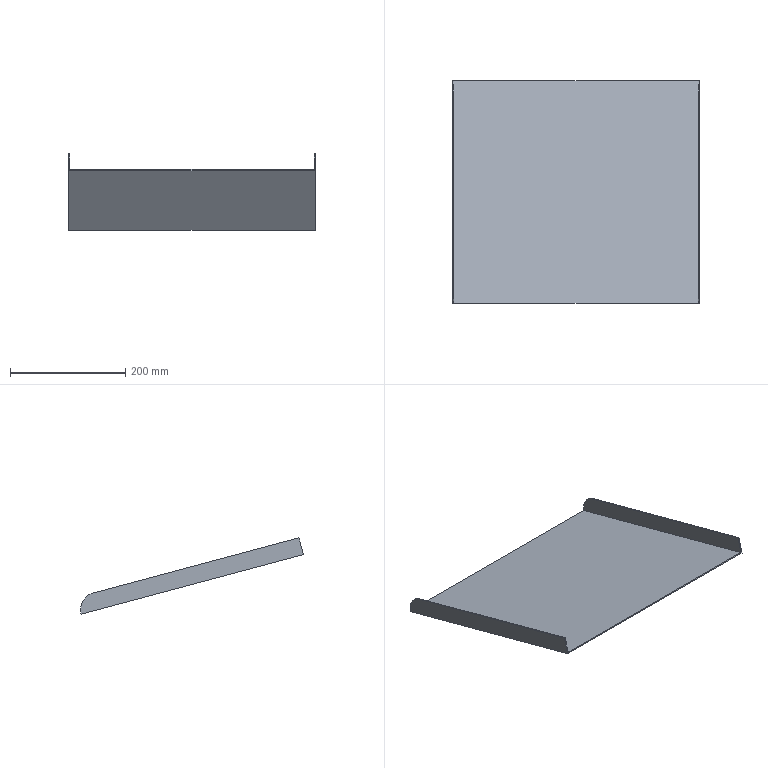Part | NX | features solid 2 | 1 solid | 12 faces | box 428.583 x 387.393 x 132.505 mm | volume 386894 mm3 | plane 10 | cylinder 2 | commonest cylinder face diameters 60 x2
STEP:
#1=CARTESIAN_POINT('',(-915.1,751.036,-491.717));
#2=VERTEX_POINT('',#1);
#3=CARTESIAN_POINT('',(-915.1,1137.342,-595.228));
#4=VERTEX_POINT('',#3);
#5=CARTESIAN_POINT('',(-915.1,973.199,-551.246));
#6=DIRECTION('',(0.,0.9659,-0.2588));
#7=VECTOR('',#6,1000.);
#8=LINE('',#5,#7);
#9=EDGE_CURVE('',#2,#4,#8,.T.);
#10=ORIENTED_EDGE('',*,*,#9,.F.);
#11=CARTESIAN_POINT('',(-490.517,751.036,-491.717));
#12=VERTEX_POINT('',#11);
#13=CARTESIAN_POINT('',(-905.1,751.036,-491.717));
#14=DIRECTION('',(-1.,0.,0.));
#15=VECTOR('',#14,1000.);
#16=LINE('',#13,#15);
#17=EDGE_CURVE('',#2,#12,#16,.F.);
#18=ORIENTED_EDGE('',*,*,#17,.T.);
#19=CARTESIAN_POINT('',(-490.517,1137.342,-595.228));
#20=VERTEX_POINT('',#19);
#21=CARTESIAN_POINT('',(-490.517,973.199,-551.246));
#22=DIRECTION('',(0.,0.9659,-0.2588));
#23=VECTOR('',#22,1000.);
#24=LINE('',#21,#23);
#25=EDGE_CURVE('',#12,#20,#24,.T.);
#26=ORIENTED_EDGE('',*,*,#25,.T.);
#27=CARTESIAN_POINT('',(-488.517,1137.342,-595.228));
#28=VERTEX_POINT('',#27);
#29=CARTESIAN_POINT('',(-478.517,1137.342,-595.228));
#30=DIRECTION('',(1.,0.,0.));
#31=VECTOR('',#30,1000.);
#32=LINE('',#29,#31);
#33=EDGE_CURVE('',#28,#20,#32,.F.);
#34=ORIENTED_EDGE('',*,*,#33,.F.);
#35=CARTESIAN_POINT('',(-488.517,1137.407,-595.245));
#36=VERTEX_POINT('',#35);
#37=CARTESIAN_POINT('',(-488.517,973.199,-551.246));
#38=DIRECTION('',(0.,-0.9659,0.2588));
#39=VECTOR('',#38,1000.);
#40=LINE('',#37,#39);
#41=EDGE_CURVE('',#28,#36,#40,.F.);
#42=ORIENTED_EDGE('',*,*,#41,.T.);
#43=CARTESIAN_POINT('',(-917.1,1137.407,-595.245));
#44=VERTEX_POINT('',#43);
#45=CARTESIAN_POINT('',(-905.1,1137.407,-595.245));
#46=DIRECTION('',(1.,0.,0.));
#47=VECTOR('',#46,1000.);
#48=LINE('',#45,#47);
#49=EDGE_CURVE('',#44,#36,#48,.T.);
#50=ORIENTED_EDGE('',*,*,#49,.F.);
#51=CARTESIAN_POINT('',(-917.1,1137.342,-595.228));
#52=VERTEX_POINT('',#51);
#53=CARTESIAN_POINT('',(-917.1,973.199,-551.246));
#54=DIRECTION('',(0.,0.9659,-0.2588));
#55=VECTOR('',#54,1000.);
#56=LINE('',#53,#55);
#57=EDGE_CURVE('',#52,#44,#56,.T.);
#58=ORIENTED_EDGE('',*,*,#57,.F.);
#59=CARTESIAN_POINT('',(-917.1,1137.342,-595.228));
#60=DIRECTION('',(-1.,0.,0.));
#61=VECTOR('',#60,1000.);
#62=LINE('',#59,#61);
#63=EDGE_CURVE('',#4,#52,#62,.T.);
#64=ORIENTED_EDGE('',*,*,#63,.F.);
#65=EDGE_LOOP('',(#10,#18,#26,#34,#42,#50,#58,#64));
#66=FACE_BOUND('',#65,.T.);
#67=CARTESIAN_POINT('',(-905.1,973.199,-551.246));
#68=DIRECTION('',(0.,0.2588,0.9659));
#69=DIRECTION('',(1.,0.,0.));
#70=AXIS2_PLACEMENT_3D('',#67,#68,#69);
#71=PLANE('',#70);
#72=ADVANCED_FACE('',(#66),#71,.T.);
#73=ORIENTED_EDGE('',*,*,#17,.F.);
#74=CARTESIAN_POINT('',(-915.1,758.283,-464.671));
#75=VERTEX_POINT('',#74);
#76=CARTESIAN_POINT('',(-915.1,750.519,-493.649));
#77=DIRECTION('',(0.,-0.2588,-0.9659));
#78=VECTOR('',#77,1000.);
#79=LINE('',#76,#78);
#80=EDGE_CURVE('',#2,#75,#79,.F.);
#81=ORIENTED_EDGE('',*,*,#80,.T.);
#82=CARTESIAN_POINT('',(-917.1,758.283,-464.671));
#83=VERTEX_POINT('',#82);
#84=CARTESIAN_POINT('',(-905.1,758.283,-464.671));
#85=DIRECTION('',(1.,0.,0.));
#86=VECTOR('',#85,1000.);
#87=LINE('',#84,#86);
#88=EDGE_CURVE('',#83,#75,#87,.T.);
#89=ORIENTED_EDGE('',*,*,#88,.F.);
#90=CARTESIAN_POINT('',(-917.1,750.519,-493.649));
#91=VERTEX_POINT('',#90);
#92=CARTESIAN_POINT('',(-917.1,751.036,-491.717));
#93=DIRECTION('',(0.,0.2588,0.9659));
#94=VECTOR('',#93,1000.);
#95=LINE('',#92,#94);
#96=EDGE_CURVE('',#83,#91,#95,.F.);
#97=ORIENTED_EDGE('',*,*,#96,.T.);
#98=CARTESIAN_POINT('',(-488.517,750.519,-493.649));
#99=VERTEX_POINT('',#98);
#100=CARTESIAN_POINT('',(-905.1,750.519,-493.649));
#101=DIRECTION('',(-1.,0.,0.));
#102=VECTOR('',#101,1000.);
#103=LINE('',#100,#102);
#104=EDGE_CURVE('',#91,#99,#103,.F.);
#105=ORIENTED_EDGE('',*,*,#104,.T.);
#106=CARTESIAN_POINT('',(-488.517,758.283,-464.671));
#107=VERTEX_POINT('',#106);
#108=CARTESIAN_POINT('',(-488.517,751.036,-491.717));
#109=DIRECTION('',(0.,-0.2588,-0.9659));
#110=VECTOR('',#109,1000.);
#111=LINE('',#108,#110);
#112=EDGE_CURVE('',#107,#99,#111,.T.);
#113=ORIENTED_EDGE('',*,*,#112,.F.);
#114=CARTESIAN_POINT('',(-490.517,758.283,-464.671));
#115=VERTEX_POINT('',#114);
#116=CARTESIAN_POINT('',(-905.1,758.283,-464.671));
#117=DIRECTION('',(1.,0.,0.));
#118=VECTOR('',#117,1000.);
#119=LINE('',#116,#118);
#120=EDGE_CURVE('',#107,#115,#119,.F.);
#121=ORIENTED_EDGE('',*,*,#120,.T.);
#122=CARTESIAN_POINT('',(-490.517,750.519,-493.649));
#123=DIRECTION('',(0.,-0.2588,-0.9659));
#124=VECTOR('',#123,1000.);
#125=LINE('',#122,#124);
#126=EDGE_CURVE('',#12,#115,#125,.F.);
#127=ORIENTED_EDGE('',*,*,#126,.F.);
#128=EDGE_LOOP('',(#73,#81,#89,#97,#105,#113,#121,#127));
#129=FACE_BOUND('',#128,.T.);
#130=CARTESIAN_POINT('',(-905.1,751.036,-491.717));
#131=DIRECTION('',(0.,-0.9659,0.2588));
#132=DIRECTION('',(1.,0.,0.));
#133=AXIS2_PLACEMENT_3D('',#130,#131,#132);
#134=PLANE('',#133);
#135=ADVANCED_FACE('',(#129),#134,.T.);
#136=ORIENTED_EDGE('',*,*,#41,.F.);
#137=CARTESIAN_POINT('',(-488.517,1115.676,-560.434));
#138=VERTEX_POINT('',#137);
#139=CARTESIAN_POINT('',(-488.517,1107.911,-589.412));
#140=DIRECTION('',(1.,0.,0.));
#141=DIRECTION('',(0.,0.,-1.));
#142=AXIS2_PLACEMENT_3D('',#139,#140,#141);
#143=CIRCLE('',#142,30.);
#144=EDGE_CURVE('',#28,#138,#143,.T.);
#145=ORIENTED_EDGE('',*,*,#144,.T.);
#146=CARTESIAN_POINT('',(-488.517,951.468,-516.435));
#147=DIRECTION('',(0.,-0.9659,0.2588));
#148=VECTOR('',#147,1000.);
#149=LINE('',#146,#148);
#150=EDGE_CURVE('',#107,#138,#149,.F.);
#151=ORIENTED_EDGE('',*,*,#150,.F.);
#152=ORIENTED_EDGE('',*,*,#112,.T.);
#153=CARTESIAN_POINT('',(-488.517,1136.889,-597.177));
#154=VERTEX_POINT('',#153);
#155=CARTESIAN_POINT('',(-488.517,972.682,-553.177));
#156=DIRECTION('',(0.,-0.9659,0.2588));
#157=VECTOR('',#156,1000.);
#158=LINE('',#155,#157);
#159=EDGE_CURVE('',#99,#154,#158,.F.);
#160=ORIENTED_EDGE('',*,*,#159,.T.);
#161=CARTESIAN_POINT('',(-488.517,1137.407,-595.245));
#162=DIRECTION('',(0.,0.2588,0.9659));
#163=VECTOR('',#162,1000.);
#164=LINE('',#161,#163);
#165=EDGE_CURVE('',#36,#154,#164,.F.);
#166=ORIENTED_EDGE('',*,*,#165,.F.);
#167=EDGE_LOOP('',(#136,#145,#151,#152,#160,#166));
#168=FACE_BOUND('',#167,.T.);
#169=CARTESIAN_POINT('',(-488.517,973.199,-551.246));
#170=DIRECTION('',(1.,0.,0.));
#171=DIRECTION('',(0.,0.9659,-0.2588));
#172=AXIS2_PLACEMENT_3D('',#169,#170,#171);
#173=PLANE('',#172);
#174=ADVANCED_FACE('',(#168),#173,.T.);
#175=ORIENTED_EDGE('',*,*,#165,.T.);
#176=CARTESIAN_POINT('',(-917.1,1136.889,-597.177));
#177=VERTEX_POINT('',#176);
#178=CARTESIAN_POINT('',(-905.1,1136.889,-597.177));
#179=DIRECTION('',(1.,0.,0.));
#180=VECTOR('',#179,1000.);
#181=LINE('',#178,#180);
#182=EDGE_CURVE('',#177,#154,#181,.T.);
#183=ORIENTED_EDGE('',*,*,#182,.F.);
#184=CARTESIAN_POINT('',(-917.1,1137.407,-595.245));
#185=DIRECTION('',(0.,-0.2588,-0.9659));
#186=VECTOR('',#185,1000.);
#187=LINE('',#184,#186);
#188=EDGE_CURVE('',#44,#177,#187,.T.);
#189=ORIENTED_EDGE('',*,*,#188,.F.);
#190=ORIENTED_EDGE('',*,*,#49,.T.);
#191=EDGE_LOOP('',(#175,#183,#189,#190));
#192=FACE_BOUND('',#191,.T.);
#193=CARTESIAN_POINT('',(-905.1,1137.407,-595.245));
#194=DIRECTION('',(0.,-0.9659,0.2588));
#195=DIRECTION('',(1.,0.,0.));
#196=AXIS2_PLACEMENT_3D('',#193,#194,#195);
#197=PLANE('',#196);
#198=ADVANCED_FACE('',(#192),#197,.F.);
#199=ORIENTED_EDGE('',*,*,#188,.T.);
#200=CARTESIAN_POINT('',(-917.1,972.682,-553.177));
#201=DIRECTION('',(0.,0.9659,-0.2588));
#202=VECTOR('',#201,1000.);
#203=LINE('',#200,#202);
#204=EDGE_CURVE('',#91,#177,#203,.T.);
#205=ORIENTED_EDGE('',*,*,#204,.F.);
#206=ORIENTED_EDGE('',*,*,#96,.F.);
#207=CARTESIAN_POINT('',(-917.1,1115.676,-560.434));
#208=VERTEX_POINT('',#207);
#209=CARTESIAN_POINT('',(-917.1,951.468,-516.435));
#210=DIRECTION('',(0.,0.9659,-0.2588));
#211=VECTOR('',#210,1000.);
#212=LINE('',#209,#211);
#213=EDGE_CURVE('',#83,#208,#212,.T.);
#214=ORIENTED_EDGE('',*,*,#213,.T.);
#215=CARTESIAN_POINT('',(-917.1,1107.911,-589.412));
#216=DIRECTION('',(1.,0.,0.));
#217=DIRECTION('',(0.,-0.2588,-0.9659));
#218=AXIS2_PLACEMENT_3D('',#215,#216,#217);
#219=CIRCLE('',#218,30.);
#220=EDGE_CURVE('',#208,#52,#219,.F.);
#221=ORIENTED_EDGE('',*,*,#220,.T.);
#222=ORIENTED_EDGE('',*,*,#57,.T.);
#223=EDGE_LOOP('',(#199,#205,#206,#214,#221,#222));
#224=FACE_BOUND('',#223,.T.);
#225=CARTESIAN_POINT('',(-917.1,973.199,-551.246));
#226=DIRECTION('',(1.,0.,0.));
#227=DIRECTION('',(0.,0.9659,-0.2588));
#228=AXIS2_PLACEMENT_3D('',#225,#226,#227);
#229=PLANE('',#228);
#230=ADVANCED_FACE('',(#224),#229,.F.);
#231=ORIENTED_EDGE('',*,*,#159,.F.);
#232=ORIENTED_EDGE('',*,*,#104,.F.);
#233=ORIENTED_EDGE('',*,*,#204,.T.);
#234=ORIENTED_EDGE('',*,*,#182,.T.);
#235=EDGE_LOOP('',(#231,#232,#233,#234));
#236=FACE_BOUND('',#235,.T.);
#237=CARTESIAN_POINT('',(-905.1,972.682,-553.177));
#238=DIRECTION('',(0.,0.2588,0.9659));
#239=DIRECTION('',(1.,0.,0.));
#240=AXIS2_PLACEMENT_3D('',#237,#238,#239);
#241=PLANE('',#240);
#242=ADVANCED_FACE('',(#236),#241,.F.);
#243=ORIENTED_EDGE('',*,*,#150,.T.);
#244=CARTESIAN_POINT('',(-490.517,1115.676,-560.434));
#245=VERTEX_POINT('',#244);
#246=CARTESIAN_POINT('',(-478.517,1115.676,-560.434));
#247=DIRECTION('',(1.,0.,0.));
#248=VECTOR('',#247,1000.);
#249=LINE('',#246,#248);
#250=EDGE_CURVE('',#138,#245,#249,.F.);
#251=ORIENTED_EDGE('',*,*,#250,.T.);
#252=CARTESIAN_POINT('',(-490.517,951.468,-516.435));
#253=DIRECTION('',(0.,0.9659,-0.2588));
#254=VECTOR('',#253,1000.);
#255=LINE('',#252,#254);
#256=EDGE_CURVE('',#115,#245,#255,.T.);
#257=ORIENTED_EDGE('',*,*,#256,.F.);
#258=ORIENTED_EDGE('',*,*,#120,.F.);
#259=EDGE_LOOP('',(#243,#251,#257,#258));
#260=FACE_BOUND('',#259,.T.);
#261=CARTESIAN_POINT('',(-478.517,951.468,-516.435));
#262=DIRECTION('',(0.,-0.2588,-0.9659));
#263=DIRECTION('',(0.,0.9659,-0.2588));
#264=AXIS2_PLACEMENT_3D('',#261,#262,#263);
#265=PLANE('',#264);
#266=ADVANCED_FACE('',(#260),#265,.F.);
#267=ORIENTED_EDGE('',*,*,#25,.F.);
#268=ORIENTED_EDGE('',*,*,#126,.T.);
#269=ORIENTED_EDGE('',*,*,#256,.T.);
#270=CARTESIAN_POINT('',(-490.517,1107.911,-589.412));
#271=DIRECTION('',(1.,0.,0.));
#272=DIRECTION('',(0.,0.,-1.));
#273=AXIS2_PLACEMENT_3D('',#270,#271,#272);
#274=CIRCLE('',#273,30.);
#275=EDGE_CURVE('',#245,#20,#274,.F.);
#276=ORIENTED_EDGE('',*,*,#275,.T.);
#277=EDGE_LOOP('',(#267,#268,#269,#276));
#278=FACE_BOUND('',#277,.T.);
#279=CARTESIAN_POINT('',(-490.517,943.704,-545.413));
#280=DIRECTION('',(1.,0.,0.));
#281=DIRECTION('',(0.,-0.2588,-0.9659));
#282=AXIS2_PLACEMENT_3D('',#279,#280,#281);
#283=PLANE('',#282);
#284=ADVANCED_FACE('',(#278),#283,.F.);
#285=ORIENTED_EDGE('',*,*,#144,.F.);
#286=ORIENTED_EDGE('',*,*,#33,.T.);
#287=ORIENTED_EDGE('',*,*,#275,.F.);
#288=ORIENTED_EDGE('',*,*,#250,.F.);
#289=EDGE_LOOP('',(#285,#286,#287,#288));
#290=FACE_BOUND('',#289,.T.);
#291=CARTESIAN_POINT('',(-478.517,1107.911,-589.412));
#292=DIRECTION('',(1.,0.,0.));
#293=DIRECTION('',(0.,-0.2588,-0.9659));
#294=AXIS2_PLACEMENT_3D('',#291,#292,#293);
#295=CYLINDRICAL_SURFACE('',#294,30.);
#296=ADVANCED_FACE('',(#290),#295,.T.);
#297=CARTESIAN_POINT('',(-915.1,1115.676,-560.434));
#298=VERTEX_POINT('',#297);
#299=CARTESIAN_POINT('',(-915.1,951.468,-516.435));
#300=DIRECTION('',(0.,0.9659,-0.2588));
#301=VECTOR('',#300,1000.);
#302=LINE('',#299,#301);
#303=EDGE_CURVE('',#75,#298,#302,.T.);
#304=ORIENTED_EDGE('',*,*,#303,.T.);
#305=CARTESIAN_POINT('',(-917.1,1115.676,-560.434));
#306=DIRECTION('',(1.,0.,0.));
#307=VECTOR('',#306,1000.);
#308=LINE('',#305,#307);
#309=EDGE_CURVE('',#298,#208,#308,.F.);
#310=ORIENTED_EDGE('',*,*,#309,.T.);
#311=ORIENTED_EDGE('',*,*,#213,.F.);
#312=ORIENTED_EDGE('',*,*,#88,.T.);
#313=EDGE_LOOP('',(#304,#310,#311,#312));
#314=FACE_BOUND('',#313,.T.);
#315=CARTESIAN_POINT('',(-917.1,951.468,-516.435));
#316=DIRECTION('',(0.,-0.2588,-0.9659));
#317=DIRECTION('',(0.,0.9659,-0.2588));
#318=AXIS2_PLACEMENT_3D('',#315,#316,#317);
#319=PLANE('',#318);
#320=ADVANCED_FACE('',(#314),#319,.F.);
#321=ORIENTED_EDGE('',*,*,#80,.F.);
#322=ORIENTED_EDGE('',*,*,#9,.T.);
#323=CARTESIAN_POINT('',(-915.1,1107.911,-589.412));
#324=DIRECTION('',(1.,0.,0.));
#325=DIRECTION('',(0.,-0.2588,-0.9659));
#326=AXIS2_PLACEMENT_3D('',#323,#324,#325);
#327=CIRCLE('',#326,30.);
#328=EDGE_CURVE('',#4,#298,#327,.T.);
#329=ORIENTED_EDGE('',*,*,#328,.T.);
#330=ORIENTED_EDGE('',*,*,#303,.F.);
#331=EDGE_LOOP('',(#321,#322,#329,#330));
#332=FACE_BOUND('',#331,.T.);
#333=CARTESIAN_POINT('',(-915.1,943.704,-545.413));
#334=DIRECTION('',(1.,0.,0.));
#335=DIRECTION('',(0.,-0.2588,-0.9659));
#336=AXIS2_PLACEMENT_3D('',#333,#334,#335);
#337=PLANE('',#336);
#338=ADVANCED_FACE('',(#332),#337,.T.);
#339=ORIENTED_EDGE('',*,*,#328,.F.);
#340=ORIENTED_EDGE('',*,*,#63,.T.);
#341=ORIENTED_EDGE('',*,*,#220,.F.);
#342=ORIENTED_EDGE('',*,*,#309,.F.);
#343=EDGE_LOOP('',(#339,#340,#341,#342));
#344=FACE_BOUND('',#343,.T.);
#345=CARTESIAN_POINT('',(-917.1,1107.911,-589.412));
#346=DIRECTION('',(-1.,0.,0.));
#347=DIRECTION('',(0.,0.2588,0.9659));
#348=AXIS2_PLACEMENT_3D('',#345,#346,#347);
#349=CYLINDRICAL_SURFACE('',#348,30.);
#350=ADVANCED_FACE('',(#344),#349,.T.);
#351=CLOSED_SHELL('',(#72,#135,#174,#198,#230,#242,#266,#284,#296,#320,#338,#350));
#352=MANIFOLD_SOLID_BREP('',#351);
#353=(LENGTH_UNIT()NAMED_UNIT(*)SI_UNIT(.MILLI.,.METRE.));
#354=UNCERTAINTY_MEASURE_WITH_UNIT(LENGTH_MEASURE(0.00001),#353,'','');
#355=(NAMED_UNIT(*)PLANE_ANGLE_UNIT()SI_UNIT($,.RADIAN.));
#356=(NAMED_UNIT(*)SI_UNIT($,.STERADIAN.)SOLID_ANGLE_UNIT());
#357=(GEOMETRIC_REPRESENTATION_CONTEXT(3)GLOBAL_UNCERTAINTY_ASSIGNED_CONTEXT((#354))GLOBAL_UNIT_ASSIGNED_CONTEXT((#353,#355,#356))REPRESENTATION_CONTEXT('',''));
#358=ADVANCED_BREP_SHAPE_REPRESENTATION('',(#352),#357);